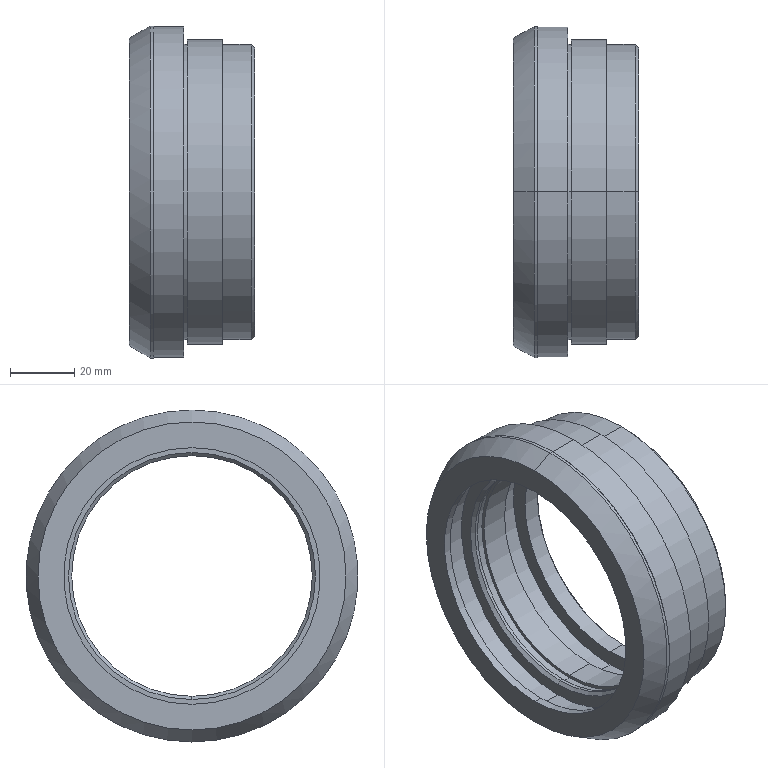Part | SolidWorks | features Chamfer 3, Revolution 1 | 1 solid | 44 faces | box 39 x 103.5 x 103.5 mm | volume 93923 mm3 | cylinder 24 | plane 12 | cone 8 | commonest cylinder face diameters 75 x6 85 x4 92 x4 77 x2 80 x2 95 x2
STEP:
#1=CARTESIAN_POINT('',(16.035,0.,-37.5));
#2=VERTEX_POINT('',#1);
#3=CARTESIAN_POINT('',(16.035,0.,37.5));
#4=VERTEX_POINT('',#3);
#5=CARTESIAN_POINT('',(16.035,0.,0.));
#6=DIRECTION('',(-1.,0.,0.));
#7=DIRECTION('',(0.,0.,-1.));
#8=AXIS2_PLACEMENT_3D('',#5,#6,#7);
#9=CIRCLE('',#8,37.5);
#10=EDGE_CURVE('',#2,#4,#9,.T.);
#11=ORIENTED_EDGE('',*,*,#10,.F.);
#12=CARTESIAN_POINT('',(15.035,0.,-38.5));
#13=VERTEX_POINT('',#12);
#14=CARTESIAN_POINT('',(16.035,0.,-37.5));
#15=DIRECTION('',(-0.7071,0.,-0.7071));
#16=VECTOR('',#15,1000.);
#17=LINE('',#14,#16);
#18=EDGE_CURVE('',#2,#13,#17,.T.);
#19=ORIENTED_EDGE('',*,*,#18,.T.);
#20=CARTESIAN_POINT('',(15.035,0.,38.5));
#21=VERTEX_POINT('',#20);
#22=CARTESIAN_POINT('',(15.035,0.,0.));
#23=DIRECTION('',(1.,0.,0.));
#24=DIRECTION('',(0.,0.,-1.));
#25=AXIS2_PLACEMENT_3D('',#22,#23,#24);
#26=CIRCLE('',#25,38.5);
#27=EDGE_CURVE('',#21,#13,#26,.T.);
#28=ORIENTED_EDGE('',*,*,#27,.F.);
#29=CARTESIAN_POINT('',(16.035,0.,37.5));
#30=DIRECTION('',(-0.7071,0.,0.7071));
#31=VECTOR('',#30,1000.);
#32=LINE('',#29,#31);
#33=EDGE_CURVE('',#4,#21,#32,.T.);
#34=ORIENTED_EDGE('',*,*,#33,.F.);
#35=EDGE_LOOP('',(#11,#19,#28,#34));
#36=FACE_OUTER_BOUND('',#35,.T.);
#37=CARTESIAN_POINT('',(16.035,0.,0.));
#38=DIRECTION('',(-1.,0.,0.));
#39=DIRECTION('',(0.,0.,1.));
#40=AXIS2_PLACEMENT_3D('',#37,#38,#39);
#41=CONICAL_SURFACE('',#40,37.5,0.7854);
#42=ADVANCED_FACE('',(#36),#41,.F.);
#43=CARTESIAN_POINT('',(43.535,0.,37.5));
#44=VERTEX_POINT('',#43);
#45=CARTESIAN_POINT('',(43.535,0.,-37.5));
#46=VERTEX_POINT('',#45);
#47=CARTESIAN_POINT('',(43.535,0.,0.));
#48=DIRECTION('',(1.,0.,0.));
#49=DIRECTION('',(0.,0.,1.));
#50=AXIS2_PLACEMENT_3D('',#47,#48,#49);
#51=CIRCLE('',#50,37.5);
#52=EDGE_CURVE('',#44,#46,#51,.T.);
#53=ORIENTED_EDGE('',*,*,#52,.F.);
#54=CARTESIAN_POINT('',(44.035,0.,38.));
#55=VERTEX_POINT('',#54);
#56=CARTESIAN_POINT('',(44.035,0.,38.));
#57=DIRECTION('',(0.7071,0.,0.7071));
#58=VECTOR('',#57,1000.);
#59=LINE('',#56,#58);
#60=EDGE_CURVE('',#44,#55,#59,.T.);
#61=ORIENTED_EDGE('',*,*,#60,.T.);
#62=CARTESIAN_POINT('',(44.035,0.,-38.));
#63=VERTEX_POINT('',#62);
#64=CARTESIAN_POINT('',(44.035,0.,0.));
#65=DIRECTION('',(-1.,0.,0.));
#66=DIRECTION('',(0.,0.,1.));
#67=AXIS2_PLACEMENT_3D('',#64,#65,#66);
#68=CIRCLE('',#67,38.);
#69=EDGE_CURVE('',#63,#55,#68,.T.);
#70=ORIENTED_EDGE('',*,*,#69,.F.);
#71=CARTESIAN_POINT('',(44.035,0.,-38.));
#72=DIRECTION('',(0.7071,0.,-0.7071));
#73=VECTOR('',#72,1000.);
#74=LINE('',#71,#73);
#75=EDGE_CURVE('',#46,#63,#74,.T.);
#76=ORIENTED_EDGE('',*,*,#75,.F.);
#77=EDGE_LOOP('',(#53,#61,#70,#76));
#78=FACE_OUTER_BOUND('',#77,.T.);
#79=CARTESIAN_POINT('',(44.035,0.,0.));
#80=DIRECTION('',(1.,0.,0.));
#81=DIRECTION('',(0.,0.,-1.));
#82=AXIS2_PLACEMENT_3D('',#79,#80,#81);
#83=CONICAL_SURFACE('',#82,38.,0.7854);
#84=ADVANCED_FACE('',(#78),#83,.F.);
#85=CARTESIAN_POINT('',(44.035,0.,-45.));
#86=VERTEX_POINT('',#85);
#87=CARTESIAN_POINT('',(44.035,0.,45.));
#88=VERTEX_POINT('',#87);
#89=CARTESIAN_POINT('',(44.035,0.,0.));
#90=DIRECTION('',(1.,0.,0.));
#91=DIRECTION('',(0.,0.,1.));
#92=AXIS2_PLACEMENT_3D('',#89,#90,#91);
#93=CIRCLE('',#92,45.);
#94=EDGE_CURVE('',#86,#88,#93,.T.);
#95=ORIENTED_EDGE('',*,*,#94,.F.);
#96=CARTESIAN_POINT('',(43.035,0.,-46.));
#97=VERTEX_POINT('',#96);
#98=CARTESIAN_POINT('',(43.035,0.,-46.));
#99=DIRECTION('',(-0.7071,0.,-0.7071));
#100=VECTOR('',#99,1000.);
#101=LINE('',#98,#100);
#102=EDGE_CURVE('',#86,#97,#101,.T.);
#103=ORIENTED_EDGE('',*,*,#102,.T.);
#104=CARTESIAN_POINT('',(43.035,0.,46.));
#105=VERTEX_POINT('',#104);
#106=CARTESIAN_POINT('',(43.035,0.,0.));
#107=DIRECTION('',(-1.,0.,0.));
#108=DIRECTION('',(0.,0.,1.));
#109=AXIS2_PLACEMENT_3D('',#106,#107,#108);
#110=CIRCLE('',#109,46.);
#111=EDGE_CURVE('',#105,#97,#110,.T.);
#112=ORIENTED_EDGE('',*,*,#111,.F.);
#113=CARTESIAN_POINT('',(43.035,0.,46.));
#114=DIRECTION('',(-0.7071,0.,0.7071));
#115=VECTOR('',#114,1000.);
#116=LINE('',#113,#115);
#117=EDGE_CURVE('',#88,#105,#116,.T.);
#118=ORIENTED_EDGE('',*,*,#117,.F.);
#119=EDGE_LOOP('',(#95,#103,#112,#118));
#120=FACE_OUTER_BOUND('',#119,.T.);
#121=CARTESIAN_POINT('',(43.035,0.,0.));
#122=DIRECTION('',(-1.,0.,0.));
#123=DIRECTION('',(0.,0.,1.));
#124=AXIS2_PLACEMENT_3D('',#121,#122,#123);
#125=CONICAL_SURFACE('',#124,46.,0.7854);
#126=ADVANCED_FACE('',(#120),#125,.T.);
#127=CARTESIAN_POINT('',(5.035,0.,48.));
#128=VERTEX_POINT('',#127);
#129=CARTESIAN_POINT('',(5.035,0.,-48.));
#130=VERTEX_POINT('',#129);
#131=CARTESIAN_POINT('',(5.035,0.,0.));
#132=DIRECTION('',(-1.,0.,0.));
#133=DIRECTION('',(0.,0.,1.));
#134=AXIS2_PLACEMENT_3D('',#131,#132,#133);
#135=CIRCLE('',#134,48.);
#136=EDGE_CURVE('',#128,#130,#135,.T.);
#137=ORIENTED_EDGE('',*,*,#136,.F.);
#138=CARTESIAN_POINT('',(11.535,0.,51.75));
#139=VERTEX_POINT('',#138);
#140=CARTESIAN_POINT('',(11.535,0.,51.75));
#141=DIRECTION('',(0.8662,0.,0.4997));
#142=VECTOR('',#141,1000.);
#143=LINE('',#140,#142);
#144=EDGE_CURVE('',#128,#139,#143,.T.);
#145=ORIENTED_EDGE('',*,*,#144,.T.);
#146=CARTESIAN_POINT('',(11.535,0.,-51.75));
#147=VERTEX_POINT('',#146);
#148=CARTESIAN_POINT('',(11.535,0.,0.));
#149=DIRECTION('',(-1.,0.,0.));
#150=DIRECTION('',(0.,0.,1.));
#151=AXIS2_PLACEMENT_3D('',#148,#149,#150);
#152=CIRCLE('',#151,51.75);
#153=EDGE_CURVE('',#139,#147,#152,.T.);
#154=ORIENTED_EDGE('',*,*,#153,.T.);
#155=CARTESIAN_POINT('',(11.535,0.,-51.75));
#156=DIRECTION('',(0.8662,0.,-0.4997));
#157=VECTOR('',#156,1000.);
#158=LINE('',#155,#157);
#159=EDGE_CURVE('',#130,#147,#158,.T.);
#160=ORIENTED_EDGE('',*,*,#159,.F.);
#161=EDGE_LOOP('',(#137,#145,#154,#160));
#162=FACE_OUTER_BOUND('',#161,.T.);
#163=CARTESIAN_POINT('',(11.535,0.,0.));
#164=DIRECTION('',(1.,0.,0.));
#165=DIRECTION('',(0.,0.,-1.));
#166=AXIS2_PLACEMENT_3D('',#163,#164,#165);
#167=CONICAL_SURFACE('',#166,51.75,0.5233);
#168=ADVANCED_FACE('',(#162),#167,.T.);
#169=CARTESIAN_POINT('',(12.535,0.,51.75));
#170=VERTEX_POINT('',#169);
#171=CARTESIAN_POINT('',(12.535,0.,-51.75));
#172=VERTEX_POINT('',#171);
#173=CARTESIAN_POINT('',(12.535,0.,0.));
#174=DIRECTION('',(-1.,0.,0.));
#175=DIRECTION('',(0.,0.,1.));
#176=AXIS2_PLACEMENT_3D('',#173,#174,#175);
#177=CIRCLE('',#176,51.75);
#178=EDGE_CURVE('',#170,#172,#177,.T.);
#179=ORIENTED_EDGE('',*,*,#178,.T.);
#180=CARTESIAN_POINT('',(-85.103,0.,-51.75));
#181=DIRECTION('',(-1.,0.,0.));
#182=VECTOR('',#181,1000.);
#183=LINE('',#180,#182);
#184=EDGE_CURVE('',#172,#147,#183,.T.);
#185=ORIENTED_EDGE('',*,*,#184,.T.);
#186=ORIENTED_EDGE('',*,*,#153,.F.);
#187=CARTESIAN_POINT('',(-85.103,0.,51.75));
#188=DIRECTION('',(-1.,0.,0.));
#189=VECTOR('',#188,1000.);
#190=LINE('',#187,#189);
#191=EDGE_CURVE('',#170,#139,#190,.T.);
#192=ORIENTED_EDGE('',*,*,#191,.F.);
#193=EDGE_LOOP('',(#179,#185,#186,#192));
#194=FACE_OUTER_BOUND('',#193,.T.);
#195=CARTESIAN_POINT('',(-85.103,0.,0.));
#196=DIRECTION('',(-1.,0.,0.));
#197=DIRECTION('',(0.,0.,1.));
#198=AXIS2_PLACEMENT_3D('',#195,#196,#197);
#199=CYLINDRICAL_SURFACE('',#198,51.75);
#200=ADVANCED_FACE('',(#194),#199,.T.);
#201=CARTESIAN_POINT('',(22.035,0.,51.5));
#202=VERTEX_POINT('',#201);
#203=CARTESIAN_POINT('',(22.035,0.,-51.5));
#204=VERTEX_POINT('',#203);
#205=CARTESIAN_POINT('',(22.035,0.,0.));
#206=DIRECTION('',(-1.,0.,0.));
#207=DIRECTION('',(0.,0.,1.));
#208=AXIS2_PLACEMENT_3D('',#205,#206,#207);
#209=CIRCLE('',#208,51.5);
#210=EDGE_CURVE('',#202,#204,#209,.T.);
#211=ORIENTED_EDGE('',*,*,#210,.T.);
#212=CARTESIAN_POINT('',(12.535,0.,-51.5));
#213=VERTEX_POINT('',#212);
#214=CARTESIAN_POINT('',(-85.103,0.,-51.5));
#215=DIRECTION('',(-1.,0.,0.));
#216=VECTOR('',#215,1000.);
#217=LINE('',#214,#216);
#218=EDGE_CURVE('',#204,#213,#217,.T.);
#219=ORIENTED_EDGE('',*,*,#218,.T.);
#220=CARTESIAN_POINT('',(12.535,0.,51.5));
#221=VERTEX_POINT('',#220);
#222=CARTESIAN_POINT('',(12.535,0.,0.));
#223=DIRECTION('',(-1.,0.,0.));
#224=DIRECTION('',(0.,0.,1.));
#225=AXIS2_PLACEMENT_3D('',#222,#223,#224);
#226=CIRCLE('',#225,51.5);
#227=EDGE_CURVE('',#221,#213,#226,.T.);
#228=ORIENTED_EDGE('',*,*,#227,.F.);
#229=CARTESIAN_POINT('',(-85.103,0.,51.5));
#230=DIRECTION('',(-1.,0.,0.));
#231=VECTOR('',#230,1000.);
#232=LINE('',#229,#231);
#233=EDGE_CURVE('',#202,#221,#232,.T.);
#234=ORIENTED_EDGE('',*,*,#233,.F.);
#235=EDGE_LOOP('',(#211,#219,#228,#234));
#236=FACE_OUTER_BOUND('',#235,.T.);
#237=CARTESIAN_POINT('',(-85.103,0.,0.));
#238=DIRECTION('',(-1.,0.,0.));
#239=DIRECTION('',(0.,0.,1.));
#240=AXIS2_PLACEMENT_3D('',#237,#238,#239);
#241=CYLINDRICAL_SURFACE('',#240,51.5);
#242=ADVANCED_FACE('',(#236),#241,.T.);
#243=CARTESIAN_POINT('',(23.035,0.,46.));
#244=VERTEX_POINT('',#243);
#245=CARTESIAN_POINT('',(23.035,0.,-46.));
#246=VERTEX_POINT('',#245);
#247=CARTESIAN_POINT('',(23.035,0.,0.));
#248=DIRECTION('',(-1.,0.,0.));
#249=DIRECTION('',(0.,0.,1.));
#250=AXIS2_PLACEMENT_3D('',#247,#248,#249);
#251=CIRCLE('',#250,46.);
#252=EDGE_CURVE('',#244,#246,#251,.T.);
#253=ORIENTED_EDGE('',*,*,#252,.T.);
#254=CARTESIAN_POINT('',(22.035,0.,-46.));
#255=VERTEX_POINT('',#254);
#256=CARTESIAN_POINT('',(-85.103,0.,-46.));
#257=DIRECTION('',(-1.,0.,0.));
#258=VECTOR('',#257,1000.);
#259=LINE('',#256,#258);
#260=EDGE_CURVE('',#246,#255,#259,.T.);
#261=ORIENTED_EDGE('',*,*,#260,.T.);
#262=CARTESIAN_POINT('',(22.035,0.,46.));
#263=VERTEX_POINT('',#262);
#264=CARTESIAN_POINT('',(22.035,0.,0.));
#265=DIRECTION('',(-1.,0.,0.));
#266=DIRECTION('',(0.,0.,1.));
#267=AXIS2_PLACEMENT_3D('',#264,#265,#266);
#268=CIRCLE('',#267,46.);
#269=EDGE_CURVE('',#263,#255,#268,.T.);
#270=ORIENTED_EDGE('',*,*,#269,.F.);
#271=CARTESIAN_POINT('',(-85.103,0.,46.));
#272=DIRECTION('',(-1.,0.,0.));
#273=VECTOR('',#272,1000.);
#274=LINE('',#271,#273);
#275=EDGE_CURVE('',#244,#263,#274,.T.);
#276=ORIENTED_EDGE('',*,*,#275,.F.);
#277=EDGE_LOOP('',(#253,#261,#270,#276));
#278=FACE_OUTER_BOUND('',#277,.T.);
#279=CARTESIAN_POINT('',(-85.103,0.,0.));
#280=DIRECTION('',(-1.,0.,0.));
#281=DIRECTION('',(0.,0.,1.));
#282=AXIS2_PLACEMENT_3D('',#279,#280,#281);
#283=CYLINDRICAL_SURFACE('',#282,46.);
#284=ADVANCED_FACE('',(#278),#283,.T.);
#285=CARTESIAN_POINT('',(34.035,0.,47.5));
#286=VERTEX_POINT('',#285);
#287=CARTESIAN_POINT('',(34.035,0.,-47.5));
#288=VERTEX_POINT('',#287);
#289=CARTESIAN_POINT('',(34.035,0.,0.));
#290=DIRECTION('',(-1.,0.,0.));
#291=DIRECTION('',(0.,0.,1.));
#292=AXIS2_PLACEMENT_3D('',#289,#290,#291);
#293=CIRCLE('',#292,47.5);
#294=EDGE_CURVE('',#286,#288,#293,.T.);
#295=ORIENTED_EDGE('',*,*,#294,.T.);
#296=CARTESIAN_POINT('',(23.035,0.,-47.5));
#297=VERTEX_POINT('',#296);
#298=CARTESIAN_POINT('',(-85.103,0.,-47.5));
#299=DIRECTION('',(-1.,0.,0.));
#300=VECTOR('',#299,1000.);
#301=LINE('',#298,#300);
#302=EDGE_CURVE('',#288,#297,#301,.T.);
#303=ORIENTED_EDGE('',*,*,#302,.T.);
#304=CARTESIAN_POINT('',(23.035,0.,47.5));
#305=VERTEX_POINT('',#304);
#306=CARTESIAN_POINT('',(23.035,0.,0.));
#307=DIRECTION('',(-1.,0.,0.));
#308=DIRECTION('',(0.,0.,1.));
#309=AXIS2_PLACEMENT_3D('',#306,#307,#308);
#310=CIRCLE('',#309,47.5);
#311=EDGE_CURVE('',#305,#297,#310,.T.);
#312=ORIENTED_EDGE('',*,*,#311,.F.);
#313=CARTESIAN_POINT('',(-85.103,0.,47.5));
#314=DIRECTION('',(-1.,0.,0.));
#315=VECTOR('',#314,1000.);
#316=LINE('',#313,#315);
#317=EDGE_CURVE('',#286,#305,#316,.T.);
#318=ORIENTED_EDGE('',*,*,#317,.F.);
#319=EDGE_LOOP('',(#295,#303,#312,#318));
#320=FACE_OUTER_BOUND('',#319,.T.);
#321=CARTESIAN_POINT('',(-85.103,0.,0.));
#322=DIRECTION('',(-1.,0.,0.));
#323=DIRECTION('',(0.,0.,1.));
#324=AXIS2_PLACEMENT_3D('',#321,#322,#323);
#325=CYLINDRICAL_SURFACE('',#324,47.5);
#326=ADVANCED_FACE('',(#320),#325,.T.);
#327=ORIENTED_EDGE('',*,*,#111,.T.);
#328=CARTESIAN_POINT('',(34.035,0.,-46.));
#329=VERTEX_POINT('',#328);
#330=CARTESIAN_POINT('',(-85.103,0.,-46.));
#331=DIRECTION('',(-1.,0.,0.));
#332=VECTOR('',#331,1000.);
#333=LINE('',#330,#332);
#334=EDGE_CURVE('',#97,#329,#333,.T.);
#335=ORIENTED_EDGE('',*,*,#334,.T.);
#336=CARTESIAN_POINT('',(34.035,0.,46.));
#337=VERTEX_POINT('',#336);
#338=CARTESIAN_POINT('',(34.035,0.,0.));
#339=DIRECTION('',(-1.,0.,0.));
#340=DIRECTION('',(0.,0.,1.));
#341=AXIS2_PLACEMENT_3D('',#338,#339,#340);
#342=CIRCLE('',#341,46.);
#343=EDGE_CURVE('',#337,#329,#342,.T.);
#344=ORIENTED_EDGE('',*,*,#343,.F.);
#345=CARTESIAN_POINT('',(-85.103,0.,46.));
#346=DIRECTION('',(-1.,0.,0.));
#347=VECTOR('',#346,1000.);
#348=LINE('',#345,#347);
#349=EDGE_CURVE('',#105,#337,#348,.T.);
#350=ORIENTED_EDGE('',*,*,#349,.F.);
#351=EDGE_LOOP('',(#327,#335,#344,#350));
#352=FACE_OUTER_BOUND('',#351,.T.);
#353=CARTESIAN_POINT('',(-85.103,0.,0.));
#354=DIRECTION('',(-1.,0.,0.));
#355=DIRECTION('',(0.,0.,1.));
#356=AXIS2_PLACEMENT_3D('',#353,#354,#355);
#357=CYLINDRICAL_SURFACE('',#356,46.);
#358=ADVANCED_FACE('',(#352),#357,.T.);
#359=ORIENTED_EDGE('',*,*,#52,.T.);
#360=CARTESIAN_POINT('',(38.035,0.,-37.5));
#361=VERTEX_POINT('',#360);
#362=CARTESIAN_POINT('',(-85.103,0.,-37.5));
#363=DIRECTION('',(-1.,0.,0.));
#364=VECTOR('',#363,1000.);
#365=LINE('',#362,#364);
#366=EDGE_CURVE('',#46,#361,#365,.T.);
#367=ORIENTED_EDGE('',*,*,#366,.T.);
#368=CARTESIAN_POINT('',(38.035,0.,37.5));
#369=VERTEX_POINT('',#368);
#370=CARTESIAN_POINT('',(38.035,0.,0.));
#371=DIRECTION('',(-1.,0.,0.));
#372=DIRECTION('',(0.,0.,1.));
#373=AXIS2_PLACEMENT_3D('',#370,#371,#372);
#374=CIRCLE('',#373,37.5);
#375=EDGE_CURVE('',#361,#369,#374,.T.);
#376=ORIENTED_EDGE('',*,*,#375,.T.);
#377=CARTESIAN_POINT('',(-85.103,0.,37.5));
#378=DIRECTION('',(-1.,0.,0.));
#379=VECTOR('',#378,1000.);
#380=LINE('',#377,#379);
#381=EDGE_CURVE('',#44,#369,#380,.T.);
#382=ORIENTED_EDGE('',*,*,#381,.F.);
#383=EDGE_LOOP('',(#359,#367,#376,#382));
#384=FACE_OUTER_BOUND('',#383,.T.);
#385=CARTESIAN_POINT('',(-85.103,0.,0.));
#386=DIRECTION('',(-1.,0.,0.));
#387=DIRECTION('',(0.,0.,1.));
#388=AXIS2_PLACEMENT_3D('',#385,#386,#387);
#389=CYLINDRICAL_SURFACE('',#388,37.5);
#390=ADVANCED_FACE('',(#384),#389,.F.);
#391=CARTESIAN_POINT('',(38.035,0.,-42.5));
#392=VERTEX_POINT('',#391);
#393=CARTESIAN_POINT('',(38.035,0.,42.5));
#394=VERTEX_POINT('',#393);
#395=CARTESIAN_POINT('',(38.035,0.,0.));
#396=DIRECTION('',(-1.,0.,0.));
#397=DIRECTION('',(0.,0.,1.));
#398=AXIS2_PLACEMENT_3D('',#395,#396,#397);
#399=CIRCLE('',#398,42.5);
#400=EDGE_CURVE('',#392,#394,#399,.T.);
#401=ORIENTED_EDGE('',*,*,#400,.F.);
#402=CARTESIAN_POINT('',(29.035,0.,-42.5));
#403=VERTEX_POINT('',#402);
#404=CARTESIAN_POINT('',(-85.103,0.,-42.5));
#405=DIRECTION('',(-1.,0.,0.));
#406=VECTOR('',#405,1000.);
#407=LINE('',#404,#406);
#408=EDGE_CURVE('',#392,#403,#407,.T.);
#409=ORIENTED_EDGE('',*,*,#408,.T.);
#410=CARTESIAN_POINT('',(29.035,0.,42.5));
#411=VERTEX_POINT('',#410);
#412=CARTESIAN_POINT('',(29.035,0.,0.));
#413=DIRECTION('',(-1.,0.,0.));
#414=DIRECTION('',(0.,0.,1.));
#415=AXIS2_PLACEMENT_3D('',#412,#413,#414);
#416=CIRCLE('',#415,42.5);
#417=EDGE_CURVE('',#403,#411,#416,.T.);
#418=ORIENTED_EDGE('',*,*,#417,.T.);
#419=CARTESIAN_POINT('',(-85.103,0.,42.5));
#420=DIRECTION('',(-1.,0.,0.));
#421=VECTOR('',#420,1000.);
#422=LINE('',#419,#421);
#423=EDGE_CURVE('',#394,#411,#422,.T.);
#424=ORIENTED_EDGE('',*,*,#423,.F.);
#425=EDGE_LOOP('',(#401,#409,#418,#424));
#426=FACE_OUTER_BOUND('',#425,.T.);
#427=CARTESIAN_POINT('',(-85.103,0.,0.));
#428=DIRECTION('',(-1.,0.,0.));
#429=DIRECTION('',(0.,0.,1.));
#430=AXIS2_PLACEMENT_3D('',#427,#428,#429);
#431=CYLINDRICAL_SURFACE('',#430,42.5);
#432=ADVANCED_FACE('',(#426),#431,.F.);
#433=CARTESIAN_POINT('',(29.035,0.,-37.5));
#434=VERTEX_POINT('',#433);
#435=CARTESIAN_POINT('',(29.035,0.,37.5));
#436=VERTEX_POINT('',#435);
#437=CARTESIAN_POINT('',(29.035,0.,0.));
#438=DIRECTION('',(-1.,0.,0.));
#439=DIRECTION('',(0.,0.,1.));
#440=AXIS2_PLACEMENT_3D('',#437,#438,#439);
#441=CIRCLE('',#440,37.5);
#442=EDGE_CURVE('',#434,#436,#441,.T.);
#443=ORIENTED_EDGE('',*,*,#442,.F.);
#444=CARTESIAN_POINT('',(20.035,0.,-37.5));
#445=VERTEX_POINT('',#444);
#446=CARTESIAN_POINT('',(-85.103,0.,-37.5));
#447=DIRECTION('',(-1.,0.,0.));
#448=VECTOR('',#447,1000.);
#449=LINE('',#446,#448);
#450=EDGE_CURVE('',#434,#445,#449,.T.);
#451=ORIENTED_EDGE('',*,*,#450,.T.);
#452=CARTESIAN_POINT('',(20.035,0.,37.5));
#453=VERTEX_POINT('',#452);
#454=CARTESIAN_POINT('',(20.035,0.,0.));
#455=DIRECTION('',(-1.,0.,0.));
#456=DIRECTION('',(0.,0.,1.));
#457=AXIS2_PLACEMENT_3D('',#454,#455,#456);
#458=CIRCLE('',#457,37.5);
#459=EDGE_CURVE('',#445,#453,#458,.T.);
#460=ORIENTED_EDGE('',*,*,#459,.T.);
#461=CARTESIAN_POINT('',(-85.103,0.,37.5));
#462=DIRECTION('',(-1.,0.,0.));
#463=VECTOR('',#462,1000.);
#464=LINE('',#461,#463);
#465=EDGE_CURVE('',#436,#453,#464,.T.);
#466=ORIENTED_EDGE('',*,*,#465,.F.);
#467=EDGE_LOOP('',(#443,#451,#460,#466));
#468=FACE_OUTER_BOUND('',#467,.T.);
#469=CARTESIAN_POINT('',(-85.103,0.,0.));
#470=DIRECTION('',(-1.,0.,0.));
#471=DIRECTION('',(0.,0.,1.));
#472=AXIS2_PLACEMENT_3D('',#469,#470,#471);
#473=CYLINDRICAL_SURFACE('',#472,37.5);
#474=ADVANCED_FACE('',(#468),#473,.F.);
#475=CARTESIAN_POINT('',(20.035,0.,-38.5));
#476=VERTEX_POINT('',#475);
#477=CARTESIAN_POINT('',(20.035,0.,38.5));
#478=VERTEX_POINT('',#477);
#479=CARTESIAN_POINT('',(20.035,0.,0.));
#480=DIRECTION('',(-1.,0.,0.));
#481=DIRECTION('',(0.,0.,1.));
#482=AXIS2_PLACEMENT_3D('',#479,#480,#481);
#483=CIRCLE('',#482,38.5);
#484=EDGE_CURVE('',#476,#478,#483,.T.);
#485=ORIENTED_EDGE('',*,*,#484,.F.);
#486=CARTESIAN_POINT('',(17.035,0.,-38.5));
#487=VERTEX_POINT('',#486);
#488=CARTESIAN_POINT('',(-85.103,0.,-38.5));
#489=DIRECTION('',(-1.,0.,0.));
#490=VECTOR('',#489,1000.);
#491=LINE('',#488,#490);
#492=EDGE_CURVE('',#476,#487,#491,.T.);
#493=ORIENTED_EDGE('',*,*,#492,.T.);
#494=CARTESIAN_POINT('',(17.035,0.,38.5));
#495=VERTEX_POINT('',#494);
#496=CARTESIAN_POINT('',(17.035,0.,0.));
#497=DIRECTION('',(-1.,0.,0.));
#498=DIRECTION('',(0.,0.,1.));
#499=AXIS2_PLACEMENT_3D('',#496,#497,#498);
#500=CIRCLE('',#499,38.5);
#501=EDGE_CURVE('',#487,#495,#500,.T.);
#502=ORIENTED_EDGE('',*,*,#501,.T.);
#503=CARTESIAN_POINT('',(-85.103,0.,38.5));
#504=DIRECTION('',(-1.,0.,0.));
#505=VECTOR('',#504,1000.);
#506=LINE('',#503,#505);
#507=EDGE_CURVE('',#478,#495,#506,.T.);
#508=ORIENTED_EDGE('',*,*,#507,.F.);
#509=EDGE_LOOP('',(#485,#493,#502,#508));
#510=FACE_OUTER_BOUND('',#509,.T.);
#511=CARTESIAN_POINT('',(-85.103,0.,0.));
#512=DIRECTION('',(-1.,0.,0.));
#513=DIRECTION('',(0.,0.,1.));
#514=AXIS2_PLACEMENT_3D('',#511,#512,#513);
#515=CYLINDRICAL_SURFACE('',#514,38.5);
#516=ADVANCED_FACE('',(#510),#515,.F.);
#517=CARTESIAN_POINT('',(17.035,0.,-37.5));
#518=VERTEX_POINT('',#517);
#519=CARTESIAN_POINT('',(17.035,0.,37.5));
#520=VERTEX_POINT('',#519);
#521=CARTESIAN_POINT('',(17.035,0.,0.));
#522=DIRECTION('',(-1.,0.,0.));
#523=DIRECTION('',(0.,0.,1.));
#524=AXIS2_PLACEMENT_3D('',#521,#522,#523);
#525=CIRCLE('',#524,37.5);
#526=EDGE_CURVE('',#518,#520,#525,.T.);
#527=ORIENTED_EDGE('',*,*,#526,.F.);
#528=CARTESIAN_POINT('',(-85.103,0.,-37.5));
#529=DIRECTION('',(-1.,0.,0.));
#530=VECTOR('',#529,1000.);
#531=LINE('',#528,#530);
#532=EDGE_CURVE('',#518,#2,#531,.T.);
#533=ORIENTED_EDGE('',*,*,#532,.T.);
#534=ORIENTED_EDGE('',*,*,#10,.T.);
#535=CARTESIAN_POINT('',(-85.103,0.,37.5));
#536=DIRECTION('',(-1.,0.,0.));
#537=VECTOR('',#536,1000.);
#538=LINE('',#535,#537);
#539=EDGE_CURVE('',#520,#4,#538,.T.);
#540=ORIENTED_EDGE('',*,*,#539,.F.);
#541=EDGE_LOOP('',(#527,#533,#534,#540));
#542=FACE_OUTER_BOUND('',#541,.T.);
#543=CARTESIAN_POINT('',(-85.103,0.,0.));
#544=DIRECTION('',(-1.,0.,0.));
#545=DIRECTION('',(0.,0.,1.));
#546=AXIS2_PLACEMENT_3D('',#543,#544,#545);
#547=CYLINDRICAL_SURFACE('',#546,37.5);
#548=ADVANCED_FACE('',(#542),#547,.F.);
#549=CARTESIAN_POINT('',(15.035,0.,-42.5));
#550=VERTEX_POINT('',#549);
#551=CARTESIAN_POINT('',(15.035,0.,42.5));
#552=VERTEX_POINT('',#551);
#553=CARTESIAN_POINT('',(15.035,0.,0.));
#554=DIRECTION('',(-1.,0.,0.));
#555=DIRECTION('',(0.,0.,1.));
#556=AXIS2_PLACEMENT_3D('',#553,#554,#555);
#557=CIRCLE('',#556,42.5);
#558=EDGE_CURVE('',#550,#552,#557,.T.);
#559=ORIENTED_EDGE('',*,*,#558,.F.);
#560=CARTESIAN_POINT('',(7.535,0.,-42.5));
#561=VERTEX_POINT('',#560);
#562=CARTESIAN_POINT('',(-85.103,0.,-42.5));
#563=DIRECTION('',(-1.,0.,0.));
#564=VECTOR('',#563,1000.);
#565=LINE('',#562,#564);
#566=EDGE_CURVE('',#550,#561,#565,.T.);
#567=ORIENTED_EDGE('',*,*,#566,.T.);
#568=CARTESIAN_POINT('',(7.535,0.,42.5));
#569=VERTEX_POINT('',#568);
#570=CARTESIAN_POINT('',(7.535,0.,0.));
#571=DIRECTION('',(-1.,0.,0.));
#572=DIRECTION('',(0.,0.,1.));
#573=AXIS2_PLACEMENT_3D('',#570,#571,#572);
#574=CIRCLE('',#573,42.5);
#575=EDGE_CURVE('',#561,#569,#574,.T.);
#576=ORIENTED_EDGE('',*,*,#575,.T.);
#577=CARTESIAN_POINT('',(-85.103,0.,42.5));
#578=DIRECTION('',(-1.,0.,0.));
#579=VECTOR('',#578,1000.);
#580=LINE('',#577,#579);
#581=EDGE_CURVE('',#552,#569,#580,.T.);
#582=ORIENTED_EDGE('',*,*,#581,.F.);
#583=EDGE_LOOP('',(#559,#567,#576,#582));
#584=FACE_OUTER_BOUND('',#583,.T.);
#585=CARTESIAN_POINT('',(-85.103,0.,0.));
#586=DIRECTION('',(-1.,0.,0.));
#587=DIRECTION('',(0.,0.,1.));
#588=AXIS2_PLACEMENT_3D('',#585,#586,#587);
#589=CYLINDRICAL_SURFACE('',#588,42.5);
#590=ADVANCED_FACE('',(#584),#589,.F.);
#591=CARTESIAN_POINT('',(7.535,0.,-40.));
#592=VERTEX_POINT('',#591);
#593=CARTESIAN_POINT('',(7.535,0.,40.));
#594=VERTEX_POINT('',#593);
#595=CARTESIAN_POINT('',(7.535,0.,0.));
#596=DIRECTION('',(-1.,0.,0.));
#597=DIRECTION('',(0.,0.,1.));
#598=AXIS2_PLACEMENT_3D('',#595,#596,#597);
#599=CIRCLE('',#598,40.);
#600=EDGE_CURVE('',#592,#594,#599,.T.);
#601=ORIENTED_EDGE('',*,*,#600,.F.);
#602=CARTESIAN_POINT('',(5.035,0.,-40.));
#603=VERTEX_POINT('',#602);
#604=CARTESIAN_POINT('',(-85.103,0.,-40.));
#605=DIRECTION('',(-1.,0.,0.));
#606=VECTOR('',#605,1000.);
#607=LINE('',#604,#606);
#608=EDGE_CURVE('',#592,#603,#607,.T.);
#609=ORIENTED_EDGE('',*,*,#608,.T.);
#610=CARTESIAN_POINT('',(5.035,0.,40.));
#611=VERTEX_POINT('',#610);
#612=CARTESIAN_POINT('',(5.035,0.,0.));
#613=DIRECTION('',(-1.,0.,0.));
#614=DIRECTION('',(0.,0.,1.));
#615=AXIS2_PLACEMENT_3D('',#612,#613,#614);
#616=CIRCLE('',#615,40.);
#617=EDGE_CURVE('',#603,#611,#616,.T.);
#618=ORIENTED_EDGE('',*,*,#617,.T.);
#619=CARTESIAN_POINT('',(-85.103,0.,40.));
#620=DIRECTION('',(-1.,0.,0.));
#621=VECTOR('',#620,1000.);
#622=LINE('',#619,#621);
#623=EDGE_CURVE('',#594,#611,#622,.T.);
#624=ORIENTED_EDGE('',*,*,#623,.F.);
#625=EDGE_LOOP('',(#601,#609,#618,#624));
#626=FACE_OUTER_BOUND('',#625,.T.);
#627=CARTESIAN_POINT('',(-85.103,0.,0.));
#628=DIRECTION('',(-1.,0.,0.));
#629=DIRECTION('',(0.,0.,1.));
#630=AXIS2_PLACEMENT_3D('',#627,#628,#629);
#631=CYLINDRICAL_SURFACE('',#630,40.);
#632=ADVANCED_FACE('',(#626),#631,.F.);
#633=CARTESIAN_POINT('',(5.035,0.,0.));
#634=DIRECTION('',(-1.,0.,0.));
#635=DIRECTION('',(0.,0.,1.));
#636=AXIS2_PLACEMENT_3D('',#633,#634,#635);
#637=CIRCLE('',#636,40.);
#638=EDGE_CURVE('',#611,#603,#637,.T.);
#639=ORIENTED_EDGE('',*,*,#638,.F.);
#640=ORIENTED_EDGE('',*,*,#617,.F.);
#641=EDGE_LOOP('',(#639,#640));
#642=FACE_BOUND('',#641,.T.);
#643=CARTESIAN_POINT('',(5.035,0.,0.));
#644=DIRECTION('',(-1.,0.,0.));
#645=DIRECTION('',(0.,0.,1.));
#646=AXIS2_PLACEMENT_3D('',#643,#644,#645);
#647=CIRCLE('',#646,48.);
#648=EDGE_CURVE('',#130,#128,#647,.T.);
#649=ORIENTED_EDGE('',*,*,#648,.T.);
#650=ORIENTED_EDGE('',*,*,#136,.T.);
#651=EDGE_LOOP('',(#649,#650));
#652=FACE_OUTER_BOUND('',#651,.T.);
#653=CARTESIAN_POINT('',(5.035,0.,-40.));
#654=DIRECTION('',(1.,0.,0.));
#655=DIRECTION('',(0.,0.,-1.));
#656=AXIS2_PLACEMENT_3D('',#653,#654,#655);
#657=PLANE('',#656);
#658=ADVANCED_FACE('',(#642,#652),#657,.F.);
#659=ORIENTED_EDGE('',*,*,#608,.F.);
#660=CARTESIAN_POINT('',(7.535,0.,0.));
#661=DIRECTION('',(-1.,0.,0.));
#662=DIRECTION('',(0.,0.,1.));
#663=AXIS2_PLACEMENT_3D('',#660,#661,#662);
#664=CIRCLE('',#663,40.);
#665=EDGE_CURVE('',#594,#592,#664,.T.);
#666=ORIENTED_EDGE('',*,*,#665,.F.);
#667=ORIENTED_EDGE('',*,*,#623,.T.);
#668=ORIENTED_EDGE('',*,*,#638,.T.);
#669=EDGE_LOOP('',(#659,#666,#667,#668));
#670=FACE_OUTER_BOUND('',#669,.T.);
#671=CARTESIAN_POINT('',(-85.103,0.,0.));
#672=DIRECTION('',(-1.,0.,0.));
#673=DIRECTION('',(0.,0.,1.));
#674=AXIS2_PLACEMENT_3D('',#671,#672,#673);
#675=CYLINDRICAL_SURFACE('',#674,40.);
#676=ADVANCED_FACE('',(#670),#675,.F.);
#677=CARTESIAN_POINT('',(7.535,0.,0.));
#678=DIRECTION('',(-1.,0.,0.));
#679=DIRECTION('',(0.,0.,1.));
#680=AXIS2_PLACEMENT_3D('',#677,#678,#679);
#681=CIRCLE('',#680,42.5);
#682=EDGE_CURVE('',#569,#561,#681,.T.);
#683=ORIENTED_EDGE('',*,*,#682,.F.);
#684=ORIENTED_EDGE('',*,*,#575,.F.);
#685=EDGE_LOOP('',(#683,#684));
#686=FACE_OUTER_BOUND('',#685,.T.);
#687=ORIENTED_EDGE('',*,*,#665,.T.);
#688=ORIENTED_EDGE('',*,*,#600,.T.);
#689=EDGE_LOOP('',(#687,#688));
#690=FACE_BOUND('',#689,.T.);
#691=CARTESIAN_POINT('',(7.535,0.,-40.));
#692=DIRECTION('',(-1.,0.,0.));
#693=DIRECTION('',(0.,0.,1.));
#694=AXIS2_PLACEMENT_3D('',#691,#692,#693);
#695=PLANE('',#694);
#696=ADVANCED_FACE('',(#686,#690),#695,.F.);
#697=ORIENTED_EDGE('',*,*,#566,.F.);
#698=CARTESIAN_POINT('',(15.035,0.,0.));
#699=DIRECTION('',(-1.,0.,0.));
#700=DIRECTION('',(0.,0.,1.));
#701=AXIS2_PLACEMENT_3D('',#698,#699,#700);
#702=CIRCLE('',#701,42.5);
#703=EDGE_CURVE('',#552,#550,#702,.T.);
#704=ORIENTED_EDGE('',*,*,#703,.F.);
#705=ORIENTED_EDGE('',*,*,#581,.T.);
#706=ORIENTED_EDGE('',*,*,#682,.T.);
#707=EDGE_LOOP('',(#697,#704,#705,#706));
#708=FACE_OUTER_BOUND('',#707,.T.);
#709=CARTESIAN_POINT('',(-85.103,0.,0.));
#710=DIRECTION('',(-1.,0.,0.));
#711=DIRECTION('',(0.,0.,1.));
#712=AXIS2_PLACEMENT_3D('',#709,#710,#711);
#713=CYLINDRICAL_SURFACE('',#712,42.5);
#714=ADVANCED_FACE('',(#708),#713,.F.);
#715=ORIENTED_EDGE('',*,*,#27,.T.);
#716=CARTESIAN_POINT('',(15.035,0.,0.));
#717=DIRECTION('',(1.,0.,0.));
#718=DIRECTION('',(0.,0.,-1.));
#719=AXIS2_PLACEMENT_3D('',#716,#717,#718);
#720=CIRCLE('',#719,38.5);
#721=EDGE_CURVE('',#13,#21,#720,.T.);
#722=ORIENTED_EDGE('',*,*,#721,.T.);
#723=EDGE_LOOP('',(#715,#722));
#724=FACE_BOUND('',#723,.T.);
#725=ORIENTED_EDGE('',*,*,#703,.T.);
#726=ORIENTED_EDGE('',*,*,#558,.T.);
#727=EDGE_LOOP('',(#725,#726));
#728=FACE_OUTER_BOUND('',#727,.T.);
#729=CARTESIAN_POINT('',(15.035,0.,-42.5));
#730=DIRECTION('',(1.,0.,0.));
#731=DIRECTION('',(0.,0.,-1.));
#732=AXIS2_PLACEMENT_3D('',#729,#730,#731);
#733=PLANE('',#732);
#734=ADVANCED_FACE('',(#724,#728),#733,.F.);
#735=ORIENTED_EDGE('',*,*,#532,.F.);
#736=CARTESIAN_POINT('',(17.035,0.,0.));
#737=DIRECTION('',(-1.,0.,0.));
#738=DIRECTION('',(0.,0.,1.));
#739=AXIS2_PLACEMENT_3D('',#736,#737,#738);
#740=CIRCLE('',#739,37.5);
#741=EDGE_CURVE('',#520,#518,#740,.T.);
#742=ORIENTED_EDGE('',*,*,#741,.F.);
#743=ORIENTED_EDGE('',*,*,#539,.T.);
#744=CARTESIAN_POINT('',(16.035,0.,0.));
#745=DIRECTION('',(-1.,0.,0.));
#746=DIRECTION('',(0.,0.,-1.));
#747=AXIS2_PLACEMENT_3D('',#744,#745,#746);
#748=CIRCLE('',#747,37.5);
#749=EDGE_CURVE('',#4,#2,#748,.T.);
#750=ORIENTED_EDGE('',*,*,#749,.T.);
#751=EDGE_LOOP('',(#735,#742,#743,#750));
#752=FACE_OUTER_BOUND('',#751,.T.);
#753=CARTESIAN_POINT('',(-85.103,0.,0.));
#754=DIRECTION('',(-1.,0.,0.));
#755=DIRECTION('',(0.,0.,1.));
#756=AXIS2_PLACEMENT_3D('',#753,#754,#755);
#757=CYLINDRICAL_SURFACE('',#756,37.5);
#758=ADVANCED_FACE('',(#752),#757,.F.);
#759=CARTESIAN_POINT('',(17.035,0.,0.));
#760=DIRECTION('',(-1.,0.,0.));
#761=DIRECTION('',(0.,0.,1.));
#762=AXIS2_PLACEMENT_3D('',#759,#760,#761);
#763=CIRCLE('',#762,38.5);
#764=EDGE_CURVE('',#495,#487,#763,.T.);
#765=ORIENTED_EDGE('',*,*,#764,.F.);
#766=ORIENTED_EDGE('',*,*,#501,.F.);
#767=EDGE_LOOP('',(#765,#766));
#768=FACE_OUTER_BOUND('',#767,.T.);
#769=ORIENTED_EDGE('',*,*,#741,.T.);
#770=ORIENTED_EDGE('',*,*,#526,.T.);
#771=EDGE_LOOP('',(#769,#770));
#772=FACE_BOUND('',#771,.T.);
#773=CARTESIAN_POINT('',(17.035,0.,-37.5));
#774=DIRECTION('',(-1.,0.,0.));
#775=DIRECTION('',(0.,0.,1.));
#776=AXIS2_PLACEMENT_3D('',#773,#774,#775);
#777=PLANE('',#776);
#778=ADVANCED_FACE('',(#768,#772),#777,.F.);
#779=ORIENTED_EDGE('',*,*,#492,.F.);
#780=CARTESIAN_POINT('',(20.035,0.,0.));
#781=DIRECTION('',(-1.,0.,0.));
#782=DIRECTION('',(0.,0.,1.));
#783=AXIS2_PLACEMENT_3D('',#780,#781,#782);
#784=CIRCLE('',#783,38.5);
#785=EDGE_CURVE('',#478,#476,#784,.T.);
#786=ORIENTED_EDGE('',*,*,#785,.F.);
#787=ORIENTED_EDGE('',*,*,#507,.T.);
#788=ORIENTED_EDGE('',*,*,#764,.T.);
#789=EDGE_LOOP('',(#779,#786,#787,#788));
#790=FACE_OUTER_BOUND('',#789,.T.);
#791=CARTESIAN_POINT('',(-85.103,0.,0.));
#792=DIRECTION('',(-1.,0.,0.));
#793=DIRECTION('',(0.,0.,1.));
#794=AXIS2_PLACEMENT_3D('',#791,#792,#793);
#795=CYLINDRICAL_SURFACE('',#794,38.5);
#796=ADVANCED_FACE('',(#790),#795,.F.);
#797=CARTESIAN_POINT('',(20.035,0.,0.));
#798=DIRECTION('',(-1.,0.,0.));
#799=DIRECTION('',(0.,0.,1.));
#800=AXIS2_PLACEMENT_3D('',#797,#798,#799);
#801=CIRCLE('',#800,37.5);
#802=EDGE_CURVE('',#453,#445,#801,.T.);
#803=ORIENTED_EDGE('',*,*,#802,.F.);
#804=ORIENTED_EDGE('',*,*,#459,.F.);
#805=EDGE_LOOP('',(#803,#804));
#806=FACE_BOUND('',#805,.T.);
#807=ORIENTED_EDGE('',*,*,#785,.T.);
#808=ORIENTED_EDGE('',*,*,#484,.T.);
#809=EDGE_LOOP('',(#807,#808));
#810=FACE_OUTER_BOUND('',#809,.T.);
#811=CARTESIAN_POINT('',(20.035,0.,-38.5));
#812=DIRECTION('',(1.,0.,0.));
#813=DIRECTION('',(0.,0.,-1.));
#814=AXIS2_PLACEMENT_3D('',#811,#812,#813);
#815=PLANE('',#814);
#816=ADVANCED_FACE('',(#806,#810),#815,.F.);
#817=ORIENTED_EDGE('',*,*,#450,.F.);
#818=CARTESIAN_POINT('',(29.035,0.,0.));
#819=DIRECTION('',(-1.,0.,0.));
#820=DIRECTION('',(0.,0.,1.));
#821=AXIS2_PLACEMENT_3D('',#818,#819,#820);
#822=CIRCLE('',#821,37.5);
#823=EDGE_CURVE('',#436,#434,#822,.T.);
#824=ORIENTED_EDGE('',*,*,#823,.F.);
#825=ORIENTED_EDGE('',*,*,#465,.T.);
#826=ORIENTED_EDGE('',*,*,#802,.T.);
#827=EDGE_LOOP('',(#817,#824,#825,#826));
#828=FACE_OUTER_BOUND('',#827,.T.);
#829=CARTESIAN_POINT('',(-85.103,0.,0.));
#830=DIRECTION('',(-1.,0.,0.));
#831=DIRECTION('',(0.,0.,1.));
#832=AXIS2_PLACEMENT_3D('',#829,#830,#831);
#833=CYLINDRICAL_SURFACE('',#832,37.5);
#834=ADVANCED_FACE('',(#828),#833,.F.);
#835=CARTESIAN_POINT('',(29.035,0.,0.));
#836=DIRECTION('',(-1.,0.,0.));
#837=DIRECTION('',(0.,0.,1.));
#838=AXIS2_PLACEMENT_3D('',#835,#836,#837);
#839=CIRCLE('',#838,42.5);
#840=EDGE_CURVE('',#411,#403,#839,.T.);
#841=ORIENTED_EDGE('',*,*,#840,.F.);
#842=ORIENTED_EDGE('',*,*,#417,.F.);
#843=EDGE_LOOP('',(#841,#842));
#844=FACE_OUTER_BOUND('',#843,.T.);
#845=ORIENTED_EDGE('',*,*,#823,.T.);
#846=ORIENTED_EDGE('',*,*,#442,.T.);
#847=EDGE_LOOP('',(#845,#846));
#848=FACE_BOUND('',#847,.T.);
#849=CARTESIAN_POINT('',(29.035,0.,-37.5));
#850=DIRECTION('',(-1.,0.,0.));
#851=DIRECTION('',(0.,0.,1.));
#852=AXIS2_PLACEMENT_3D('',#849,#850,#851);
#853=PLANE('',#852);
#854=ADVANCED_FACE('',(#844,#848),#853,.F.);
#855=ORIENTED_EDGE('',*,*,#408,.F.);
#856=CARTESIAN_POINT('',(38.035,0.,0.));
#857=DIRECTION('',(-1.,0.,0.));
#858=DIRECTION('',(0.,0.,1.));
#859=AXIS2_PLACEMENT_3D('',#856,#857,#858);
#860=CIRCLE('',#859,42.5);
#861=EDGE_CURVE('',#394,#392,#860,.T.);
#862=ORIENTED_EDGE('',*,*,#861,.F.);
#863=ORIENTED_EDGE('',*,*,#423,.T.);
#864=ORIENTED_EDGE('',*,*,#840,.T.);
#865=EDGE_LOOP('',(#855,#862,#863,#864));
#866=FACE_OUTER_BOUND('',#865,.T.);
#867=CARTESIAN_POINT('',(-85.103,0.,0.));
#868=DIRECTION('',(-1.,0.,0.));
#869=DIRECTION('',(0.,0.,1.));
#870=AXIS2_PLACEMENT_3D('',#867,#868,#869);
#871=CYLINDRICAL_SURFACE('',#870,42.5);
#872=ADVANCED_FACE('',(#866),#871,.F.);
#873=CARTESIAN_POINT('',(38.035,0.,0.));
#874=DIRECTION('',(-1.,0.,0.));
#875=DIRECTION('',(0.,0.,1.));
#876=AXIS2_PLACEMENT_3D('',#873,#874,#875);
#877=CIRCLE('',#876,37.5);
#878=EDGE_CURVE('',#369,#361,#877,.T.);
#879=ORIENTED_EDGE('',*,*,#878,.F.);
#880=ORIENTED_EDGE('',*,*,#375,.F.);
#881=EDGE_LOOP('',(#879,#880));
#882=FACE_BOUND('',#881,.T.);
#883=ORIENTED_EDGE('',*,*,#861,.T.);
#884=ORIENTED_EDGE('',*,*,#400,.T.);
#885=EDGE_LOOP('',(#883,#884));
#886=FACE_OUTER_BOUND('',#885,.T.);
#887=CARTESIAN_POINT('',(38.035,0.,-42.5));
#888=DIRECTION('',(1.,0.,0.));
#889=DIRECTION('',(0.,0.,-1.));
#890=AXIS2_PLACEMENT_3D('',#887,#888,#889);
#891=PLANE('',#890);
#892=ADVANCED_FACE('',(#882,#886),#891,.F.);
#893=ORIENTED_EDGE('',*,*,#366,.F.);
#894=CARTESIAN_POINT('',(43.535,0.,0.));
#895=DIRECTION('',(1.,0.,0.));
#896=DIRECTION('',(0.,0.,1.));
#897=AXIS2_PLACEMENT_3D('',#894,#895,#896);
#898=CIRCLE('',#897,37.5);
#899=EDGE_CURVE('',#46,#44,#898,.T.);
#900=ORIENTED_EDGE('',*,*,#899,.T.);
#901=ORIENTED_EDGE('',*,*,#381,.T.);
#902=ORIENTED_EDGE('',*,*,#878,.T.);
#903=EDGE_LOOP('',(#893,#900,#901,#902));
#904=FACE_OUTER_BOUND('',#903,.T.);
#905=CARTESIAN_POINT('',(-85.103,0.,0.));
#906=DIRECTION('',(-1.,0.,0.));
#907=DIRECTION('',(0.,0.,1.));
#908=AXIS2_PLACEMENT_3D('',#905,#906,#907);
#909=CYLINDRICAL_SURFACE('',#908,37.5);
#910=ADVANCED_FACE('',(#904),#909,.F.);
#911=ORIENTED_EDGE('',*,*,#69,.T.);
#912=CARTESIAN_POINT('',(44.035,0.,0.));
#913=DIRECTION('',(-1.,0.,0.));
#914=DIRECTION('',(0.,0.,1.));
#915=AXIS2_PLACEMENT_3D('',#912,#913,#914);
#916=CIRCLE('',#915,38.);
#917=EDGE_CURVE('',#55,#63,#916,.T.);
#918=ORIENTED_EDGE('',*,*,#917,.T.);
#919=EDGE_LOOP('',(#911,#918));
#920=FACE_BOUND('',#919,.T.);
#921=CARTESIAN_POINT('',(44.035,0.,0.));
#922=DIRECTION('',(1.,0.,0.));
#923=DIRECTION('',(0.,0.,1.));
#924=AXIS2_PLACEMENT_3D('',#921,#922,#923);
#925=CIRCLE('',#924,45.);
#926=EDGE_CURVE('',#88,#86,#925,.T.);
#927=ORIENTED_EDGE('',*,*,#926,.T.);
#928=ORIENTED_EDGE('',*,*,#94,.T.);
#929=EDGE_LOOP('',(#927,#928));
#930=FACE_OUTER_BOUND('',#929,.T.);
#931=CARTESIAN_POINT('',(44.035,0.,-37.5));
#932=DIRECTION('',(-1.,0.,0.));
#933=DIRECTION('',(0.,0.,1.));
#934=AXIS2_PLACEMENT_3D('',#931,#932,#933);
#935=PLANE('',#934);
#936=ADVANCED_FACE('',(#920,#930),#935,.F.);
#937=ORIENTED_EDGE('',*,*,#334,.F.);
#938=CARTESIAN_POINT('',(43.035,0.,0.));
#939=DIRECTION('',(-1.,0.,0.));
#940=DIRECTION('',(0.,0.,1.));
#941=AXIS2_PLACEMENT_3D('',#938,#939,#940);
#942=CIRCLE('',#941,46.);
#943=EDGE_CURVE('',#97,#105,#942,.T.);
#944=ORIENTED_EDGE('',*,*,#943,.T.);
#945=ORIENTED_EDGE('',*,*,#349,.T.);
#946=CARTESIAN_POINT('',(34.035,0.,0.));
#947=DIRECTION('',(-1.,0.,0.));
#948=DIRECTION('',(0.,0.,1.));
#949=AXIS2_PLACEMENT_3D('',#946,#947,#948);
#950=CIRCLE('',#949,46.);
#951=EDGE_CURVE('',#329,#337,#950,.T.);
#952=ORIENTED_EDGE('',*,*,#951,.F.);
#953=EDGE_LOOP('',(#937,#944,#945,#952));
#954=FACE_OUTER_BOUND('',#953,.T.);
#955=CARTESIAN_POINT('',(-85.103,0.,0.));
#956=DIRECTION('',(-1.,0.,0.));
#957=DIRECTION('',(0.,0.,1.));
#958=AXIS2_PLACEMENT_3D('',#955,#956,#957);
#959=CYLINDRICAL_SURFACE('',#958,46.);
#960=ADVANCED_FACE('',(#954),#959,.T.);
#961=ORIENTED_EDGE('',*,*,#294,.F.);
#962=CARTESIAN_POINT('',(34.035,0.,0.));
#963=DIRECTION('',(-1.,0.,0.));
#964=DIRECTION('',(0.,0.,1.));
#965=AXIS2_PLACEMENT_3D('',#962,#963,#964);
#966=CIRCLE('',#965,47.5);
#967=EDGE_CURVE('',#288,#286,#966,.T.);
#968=ORIENTED_EDGE('',*,*,#967,.F.);
#969=EDGE_LOOP('',(#961,#968));
#970=FACE_OUTER_BOUND('',#969,.T.);
#971=ORIENTED_EDGE('',*,*,#343,.T.);
#972=ORIENTED_EDGE('',*,*,#951,.T.);
#973=EDGE_LOOP('',(#971,#972));
#974=FACE_BOUND('',#973,.T.);
#975=CARTESIAN_POINT('',(34.035,0.,-46.));
#976=DIRECTION('',(-1.,0.,0.));
#977=DIRECTION('',(0.,0.,1.));
#978=AXIS2_PLACEMENT_3D('',#975,#976,#977);
#979=PLANE('',#978);
#980=ADVANCED_FACE('',(#970,#974),#979,.F.);
#981=ORIENTED_EDGE('',*,*,#302,.F.);
#982=ORIENTED_EDGE('',*,*,#967,.T.);
#983=ORIENTED_EDGE('',*,*,#317,.T.);
#984=CARTESIAN_POINT('',(23.035,0.,0.));
#985=DIRECTION('',(-1.,0.,0.));
#986=DIRECTION('',(0.,0.,1.));
#987=AXIS2_PLACEMENT_3D('',#984,#985,#986);
#988=CIRCLE('',#987,47.5);
#989=EDGE_CURVE('',#297,#305,#988,.T.);
#990=ORIENTED_EDGE('',*,*,#989,.F.);
#991=EDGE_LOOP('',(#981,#982,#983,#990));
#992=FACE_OUTER_BOUND('',#991,.T.);
#993=CARTESIAN_POINT('',(-85.103,0.,0.));
#994=DIRECTION('',(-1.,0.,0.));
#995=DIRECTION('',(0.,0.,1.));
#996=AXIS2_PLACEMENT_3D('',#993,#994,#995);
#997=CYLINDRICAL_SURFACE('',#996,47.5);
#998=ADVANCED_FACE('',(#992),#997,.T.);
#999=ORIENTED_EDGE('',*,*,#252,.F.);
#1000=CARTESIAN_POINT('',(23.035,0.,0.));
#1001=DIRECTION('',(-1.,0.,0.));
#1002=DIRECTION('',(0.,0.,1.));
#1003=AXIS2_PLACEMENT_3D('',#1000,#1001,#1002);
#1004=CIRCLE('',#1003,46.);
#1005=EDGE_CURVE('',#246,#244,#1004,.T.);
#1006=ORIENTED_EDGE('',*,*,#1005,.F.);
#1007=EDGE_LOOP('',(#999,#1006));
#1008=FACE_BOUND('',#1007,.T.);
#1009=ORIENTED_EDGE('',*,*,#311,.T.);
#1010=ORIENTED_EDGE('',*,*,#989,.T.);
#1011=EDGE_LOOP('',(#1009,#1010));
#1012=FACE_OUTER_BOUND('',#1011,.T.);
#1013=CARTESIAN_POINT('',(23.035,0.,-47.5));
#1014=DIRECTION('',(1.,0.,0.));
#1015=DIRECTION('',(0.,0.,-1.));
#1016=AXIS2_PLACEMENT_3D('',#1013,#1014,#1015);
#1017=PLANE('',#1016);
#1018=ADVANCED_FACE('',(#1008,#1012),#1017,.F.);
#1019=ORIENTED_EDGE('',*,*,#260,.F.);
#1020=ORIENTED_EDGE('',*,*,#1005,.T.);
#1021=ORIENTED_EDGE('',*,*,#275,.T.);
#1022=CARTESIAN_POINT('',(22.035,0.,0.));
#1023=DIRECTION('',(-1.,0.,0.));
#1024=DIRECTION('',(0.,0.,1.));
#1025=AXIS2_PLACEMENT_3D('',#1022,#1023,#1024);
#1026=CIRCLE('',#1025,46.);
#1027=EDGE_CURVE('',#255,#263,#1026,.T.);
#1028=ORIENTED_EDGE('',*,*,#1027,.F.);
#1029=EDGE_LOOP('',(#1019,#1020,#1021,#1028));
#1030=FACE_OUTER_BOUND('',#1029,.T.);
#1031=CARTESIAN_POINT('',(-85.103,0.,0.));
#1032=DIRECTION('',(-1.,0.,0.));
#1033=DIRECTION('',(0.,0.,1.));
#1034=AXIS2_PLACEMENT_3D('',#1031,#1032,#1033);
#1035=CYLINDRICAL_SURFACE('',#1034,46.);
#1036=ADVANCED_FACE('',(#1030),#1035,.T.);
#1037=ORIENTED_EDGE('',*,*,#210,.F.);
#1038=CARTESIAN_POINT('',(22.035,0.,0.));
#1039=DIRECTION('',(-1.,0.,0.));
#1040=DIRECTION('',(0.,0.,1.));
#1041=AXIS2_PLACEMENT_3D('',#1038,#1039,#1040);
#1042=CIRCLE('',#1041,51.5);
#1043=EDGE_CURVE('',#204,#202,#1042,.T.);
#1044=ORIENTED_EDGE('',*,*,#1043,.F.);
#1045=EDGE_LOOP('',(#1037,#1044));
#1046=FACE_OUTER_BOUND('',#1045,.T.);
#1047=ORIENTED_EDGE('',*,*,#269,.T.);
#1048=ORIENTED_EDGE('',*,*,#1027,.T.);
#1049=EDGE_LOOP('',(#1047,#1048));
#1050=FACE_BOUND('',#1049,.T.);
#1051=CARTESIAN_POINT('',(22.035,0.,-46.));
#1052=DIRECTION('',(-1.,0.,0.));
#1053=DIRECTION('',(0.,0.,1.));
#1054=AXIS2_PLACEMENT_3D('',#1051,#1052,#1053);
#1055=PLANE('',#1054);
#1056=ADVANCED_FACE('',(#1046,#1050),#1055,.F.);
#1057=ORIENTED_EDGE('',*,*,#218,.F.);
#1058=ORIENTED_EDGE('',*,*,#1043,.T.);
#1059=ORIENTED_EDGE('',*,*,#233,.T.);
#1060=CARTESIAN_POINT('',(12.535,0.,0.));
#1061=DIRECTION('',(-1.,0.,0.));
#1062=DIRECTION('',(0.,0.,1.));
#1063=AXIS2_PLACEMENT_3D('',#1060,#1061,#1062);
#1064=CIRCLE('',#1063,51.5);
#1065=EDGE_CURVE('',#213,#221,#1064,.T.);
#1066=ORIENTED_EDGE('',*,*,#1065,.F.);
#1067=EDGE_LOOP('',(#1057,#1058,#1059,#1066));
#1068=FACE_OUTER_BOUND('',#1067,.T.);
#1069=CARTESIAN_POINT('',(-85.103,0.,0.));
#1070=DIRECTION('',(-1.,0.,0.));
#1071=DIRECTION('',(0.,0.,1.));
#1072=AXIS2_PLACEMENT_3D('',#1069,#1070,#1071);
#1073=CYLINDRICAL_SURFACE('',#1072,51.5);
#1074=ADVANCED_FACE('',(#1068),#1073,.T.);
#1075=ORIENTED_EDGE('',*,*,#178,.F.);
#1076=CARTESIAN_POINT('',(12.535,0.,0.));
#1077=DIRECTION('',(-1.,0.,0.));
#1078=DIRECTION('',(0.,0.,1.));
#1079=AXIS2_PLACEMENT_3D('',#1076,#1077,#1078);
#1080=CIRCLE('',#1079,51.75);
#1081=EDGE_CURVE('',#172,#170,#1080,.T.);
#1082=ORIENTED_EDGE('',*,*,#1081,.F.);
#1083=EDGE_LOOP('',(#1075,#1082));
#1084=FACE_OUTER_BOUND('',#1083,.T.);
#1085=ORIENTED_EDGE('',*,*,#227,.T.);
#1086=ORIENTED_EDGE('',*,*,#1065,.T.);
#1087=EDGE_LOOP('',(#1085,#1086));
#1088=FACE_BOUND('',#1087,.T.);
#1089=CARTESIAN_POINT('',(12.535,0.,-51.5));
#1090=DIRECTION('',(-1.,0.,0.));
#1091=DIRECTION('',(0.,0.,1.));
#1092=AXIS2_PLACEMENT_3D('',#1089,#1090,#1091);
#1093=PLANE('',#1092);
#1094=ADVANCED_FACE('',(#1084,#1088),#1093,.F.);
#1095=ORIENTED_EDGE('',*,*,#184,.F.);
#1096=ORIENTED_EDGE('',*,*,#1081,.T.);
#1097=ORIENTED_EDGE('',*,*,#191,.T.);
#1098=CARTESIAN_POINT('',(11.535,0.,0.));
#1099=DIRECTION('',(-1.,0.,0.));
#1100=DIRECTION('',(0.,0.,1.));
#1101=AXIS2_PLACEMENT_3D('',#1098,#1099,#1100);
#1102=CIRCLE('',#1101,51.75);
#1103=EDGE_CURVE('',#147,#139,#1102,.T.);
#1104=ORIENTED_EDGE('',*,*,#1103,.F.);
#1105=EDGE_LOOP('',(#1095,#1096,#1097,#1104));
#1106=FACE_OUTER_BOUND('',#1105,.T.);
#1107=CARTESIAN_POINT('',(-85.103,0.,0.));
#1108=DIRECTION('',(-1.,0.,0.));
#1109=DIRECTION('',(0.,0.,1.));
#1110=AXIS2_PLACEMENT_3D('',#1107,#1108,#1109);
#1111=CYLINDRICAL_SURFACE('',#1110,51.75);
#1112=ADVANCED_FACE('',(#1106),#1111,.T.);
#1113=ORIENTED_EDGE('',*,*,#144,.F.);
#1114=ORIENTED_EDGE('',*,*,#648,.F.);
#1115=ORIENTED_EDGE('',*,*,#159,.T.);
#1116=ORIENTED_EDGE('',*,*,#1103,.T.);
#1117=EDGE_LOOP('',(#1113,#1114,#1115,#1116));
#1118=FACE_OUTER_BOUND('',#1117,.T.);
#1119=CARTESIAN_POINT('',(11.535,0.,0.));
#1120=DIRECTION('',(1.,0.,0.));
#1121=DIRECTION('',(0.,0.,-1.));
#1122=AXIS2_PLACEMENT_3D('',#1119,#1120,#1121);
#1123=CONICAL_SURFACE('',#1122,51.75,0.5233);
#1124=ADVANCED_FACE('',(#1118),#1123,.T.);
#1125=ORIENTED_EDGE('',*,*,#102,.F.);
#1126=ORIENTED_EDGE('',*,*,#926,.F.);
#1127=ORIENTED_EDGE('',*,*,#117,.T.);
#1128=ORIENTED_EDGE('',*,*,#943,.F.);
#1129=EDGE_LOOP('',(#1125,#1126,#1127,#1128));
#1130=FACE_OUTER_BOUND('',#1129,.T.);
#1131=CARTESIAN_POINT('',(43.035,0.,0.));
#1132=DIRECTION('',(-1.,0.,0.));
#1133=DIRECTION('',(0.,0.,1.));
#1134=AXIS2_PLACEMENT_3D('',#1131,#1132,#1133);
#1135=CONICAL_SURFACE('',#1134,46.,0.7854);
#1136=ADVANCED_FACE('',(#1130),#1135,.T.);
#1137=ORIENTED_EDGE('',*,*,#60,.F.);
#1138=ORIENTED_EDGE('',*,*,#899,.F.);
#1139=ORIENTED_EDGE('',*,*,#75,.T.);
#1140=ORIENTED_EDGE('',*,*,#917,.F.);
#1141=EDGE_LOOP('',(#1137,#1138,#1139,#1140));
#1142=FACE_OUTER_BOUND('',#1141,.T.);
#1143=CARTESIAN_POINT('',(44.035,0.,0.));
#1144=DIRECTION('',(1.,0.,0.));
#1145=DIRECTION('',(0.,0.,-1.));
#1146=AXIS2_PLACEMENT_3D('',#1143,#1144,#1145);
#1147=CONICAL_SURFACE('',#1146,38.,0.7854);
#1148=ADVANCED_FACE('',(#1142),#1147,.F.);
#1149=ORIENTED_EDGE('',*,*,#18,.F.);
#1150=ORIENTED_EDGE('',*,*,#749,.F.);
#1151=ORIENTED_EDGE('',*,*,#33,.T.);
#1152=ORIENTED_EDGE('',*,*,#721,.F.);
#1153=EDGE_LOOP('',(#1149,#1150,#1151,#1152));
#1154=FACE_OUTER_BOUND('',#1153,.T.);
#1155=CARTESIAN_POINT('',(16.035,0.,0.));
#1156=DIRECTION('',(-1.,0.,0.));
#1157=DIRECTION('',(0.,0.,1.));
#1158=AXIS2_PLACEMENT_3D('',#1155,#1156,#1157);
#1159=CONICAL_SURFACE('',#1158,37.5,0.7854);
#1160=ADVANCED_FACE('',(#1154),#1159,.F.);
#1161=CLOSED_SHELL('',(#42,#84,#126,#168,#200,#242,#284,#326,#358,#390,#432,#474,#516,#548,#590,#632,#658,#676,#696,#714,#734,#758,#778,#796,#816,#834,#854,#872,#892,#910,#936,#960,#980,#998,#1018,#1036,#1056,#1074,#1094,#1112,#1124,#1136,#1148,#1160));
#1162=MANIFOLD_SOLID_BREP('',#1161);
#1163=CARTESIAN_POINT('',(0.,0.,0.));
#1164=DIRECTION('',(0.,0.,1.));
#1165=DIRECTION('',(1.,0.,0.));
#1166=AXIS2_PLACEMENT_3D('',#1163,#1164,#1165);
#1167=(LENGTH_UNIT()NAMED_UNIT(*)SI_UNIT(.MILLI.,.METRE.));
#1168=UNCERTAINTY_MEASURE_WITH_UNIT(LENGTH_MEASURE(0.00001),#1167,'','');
#1169=(NAMED_UNIT(*)PLANE_ANGLE_UNIT()SI_UNIT($,.RADIAN.));
#1170=(NAMED_UNIT(*)SI_UNIT($,.STERADIAN.)SOLID_ANGLE_UNIT());
#1171=(GEOMETRIC_REPRESENTATION_CONTEXT(3)GLOBAL_UNCERTAINTY_ASSIGNED_CONTEXT((#1168))GLOBAL_UNIT_ASSIGNED_CONTEXT((#1167,#1169,#1170))REPRESENTATION_CONTEXT('',''));
#1172=ADVANCED_BREP_SHAPE_REPRESENTATION('',(#1162,#1166),#1171);